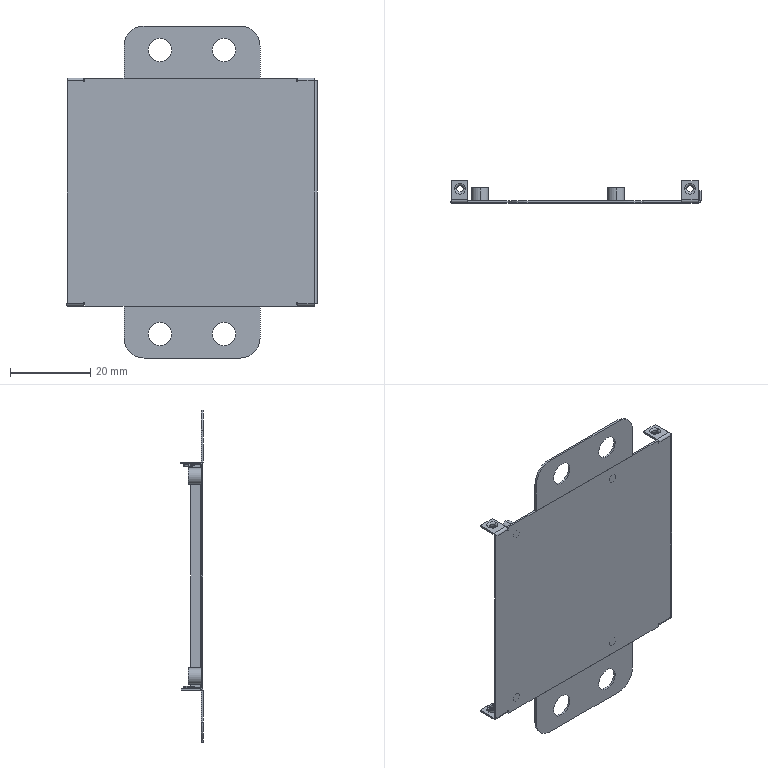Part | NX | features BREP 1 | 1 solid | 744 faces | box 62.5 x 5.5 x 83 mm | volume 2275 mm3 | spline 364 | cylinder 278 | plane 78 | torus 16 | cone 8 | commonest cylinder face diameters 2.013 x168 2.5 x64 1.7 x8 2.64 x8 4.2 x8 5.8 x8